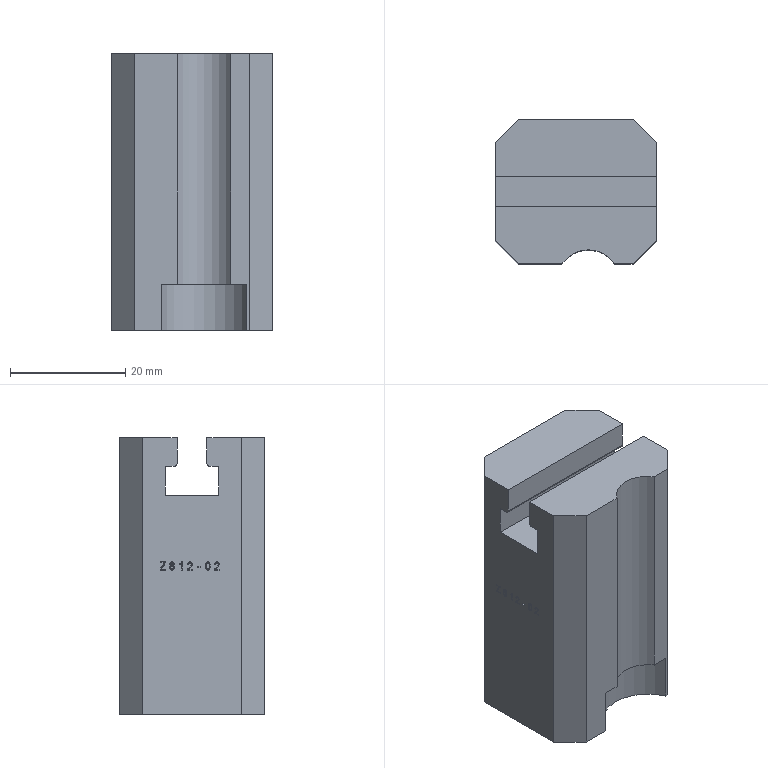Part | Creo | 1 solid | 157 faces | box 28 x 25 x 48 mm | volume 27194 mm3 | other 91 | plane 53 | cylinder 11 | cone 2 | commonest cylinder face diameters 1 x2 1.208 x2 8.499 x2 8.5 x2 11 x1 16 x1